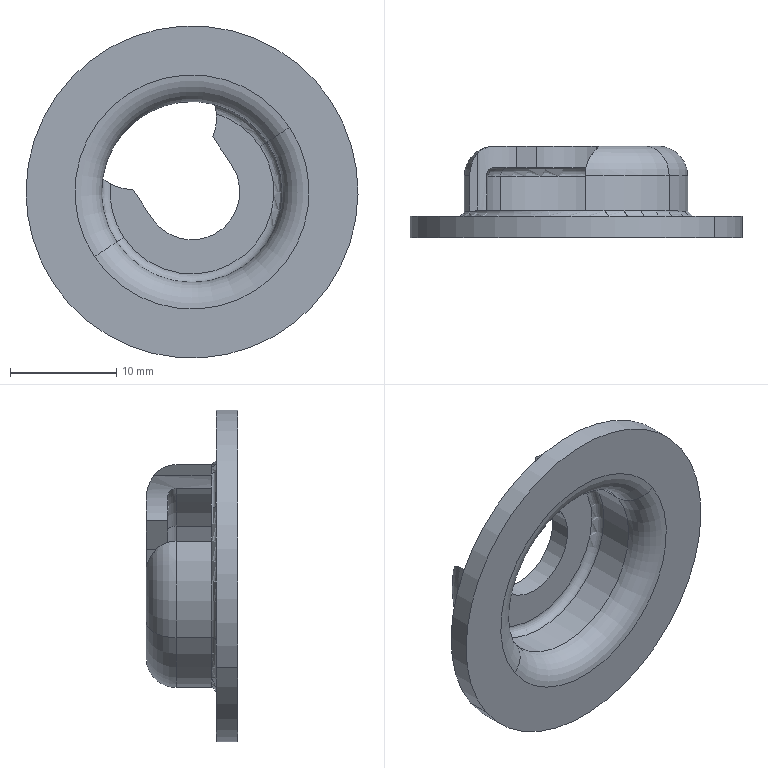Part | SolidWorks | features BaseBody 1 | 1 solid | 30 faces | box 31.2 x 8.6 x 31.2 mm | volume 1769 mm3 | cylinder 11 | torus 10 | plane 9 | commonest cylinder face diameters 9 x3 17 x3 21 x3 31.2 x2
STEP:
#1=CARTESIAN_POINT('',(45.671,49.147,6.074));
#2=VERTEX_POINT('',#1);
#3=CARTESIAN_POINT('',(27.329,49.147,-6.074));
#4=VERTEX_POINT('',#3);
#5=CARTESIAN_POINT('',(36.5,49.147,0.));
#6=DIRECTION('',(0.,1.,0.));
#7=DIRECTION('',(-0.8337,0.,-0.5522));
#8=AXIS2_PLACEMENT_3D('',#5,#6,#7);
#9=CIRCLE('',#8,11.);
#10=EDGE_CURVE('',#2,#4,#9,.T.);
#11=ORIENTED_EDGE('',*,*,#10,.F.);
#12=CARTESIAN_POINT('',(43.587,51.647,4.693));
#13=VERTEX_POINT('',#12);
#14=CARTESIAN_POINT('',(45.671,51.647,6.074));
#15=DIRECTION('',(0.5522,0.,-0.8337));
#16=DIRECTION('',(-0.8337,0.,-0.5522));
#17=AXIS2_PLACEMENT_3D('',#14,#15,#16);
#18=CIRCLE('',#17,2.5);
#19=EDGE_CURVE('',#2,#13,#18,.T.);
#20=ORIENTED_EDGE('',*,*,#19,.T.);
#21=CARTESIAN_POINT('',(29.413,51.647,-4.693));
#22=VERTEX_POINT('',#21);
#23=CARTESIAN_POINT('',(36.5,51.647,0.));
#24=DIRECTION('',(0.,-1.,0.));
#25=DIRECTION('',(-0.8337,0.,-0.5522));
#26=AXIS2_PLACEMENT_3D('',#23,#24,#25);
#27=CIRCLE('',#26,8.5);
#28=EDGE_CURVE('',#22,#13,#27,.T.);
#29=ORIENTED_EDGE('',*,*,#28,.F.);
#30=CARTESIAN_POINT('',(27.329,51.647,-6.074));
#31=DIRECTION('',(-0.5522,0.,0.8337));
#32=DIRECTION('',(0.8337,0.,0.5522));
#33=AXIS2_PLACEMENT_3D('',#30,#31,#32);
#34=CIRCLE('',#33,2.5);
#35=EDGE_CURVE('',#4,#22,#34,.T.);
#36=ORIENTED_EDGE('',*,*,#35,.F.);
#37=EDGE_LOOP('',(#11,#20,#29,#36));
#38=FACE_OUTER_BOUND('',#37,.T.);
#39=CARTESIAN_POINT('',(36.5,51.647,0.));
#40=DIRECTION('',(0.,-1.,0.));
#41=DIRECTION('',(-0.8337,0.,-0.5522));
#42=AXIS2_PLACEMENT_3D('',#39,#40,#41);
#43=TOROIDAL_SURFACE('',#42,11.,2.5);
#44=ADVANCED_FACE('',(#38),#43,.T.);
#45=CARTESIAN_POINT('',(45.671,51.147,6.074));
#46=VERTEX_POINT('',#45);
#47=CARTESIAN_POINT('',(27.329,51.147,-6.074));
#48=VERTEX_POINT('',#47);
#49=CARTESIAN_POINT('',(36.5,51.147,0.));
#50=DIRECTION('',(0.,-1.,0.));
#51=DIRECTION('',(-0.8337,0.,-0.5522));
#52=AXIS2_PLACEMENT_3D('',#49,#50,#51);
#53=CIRCLE('',#52,11.);
#54=EDGE_CURVE('',#46,#48,#53,.T.);
#55=ORIENTED_EDGE('',*,*,#54,.F.);
#56=CARTESIAN_POINT('',(45.254,51.647,5.798));
#57=VERTEX_POINT('',#56);
#58=CARTESIAN_POINT('',(45.671,51.647,6.074));
#59=DIRECTION('',(0.5522,0.,-0.8337));
#60=DIRECTION('',(-0.8337,0.,-0.5522));
#61=AXIS2_PLACEMENT_3D('',#58,#59,#60);
#62=CIRCLE('',#61,0.5);
#63=EDGE_CURVE('',#46,#57,#62,.T.);
#64=ORIENTED_EDGE('',*,*,#63,.T.);
#65=CARTESIAN_POINT('',(37.366,51.647,10.464));
#66=VERTEX_POINT('',#65);
#67=CARTESIAN_POINT('',(36.5,51.647,0.));
#68=DIRECTION('',(0.,1.,0.));
#69=DIRECTION('',(-0.8337,0.,-0.5522));
#70=AXIS2_PLACEMENT_3D('',#67,#68,#69);
#71=CIRCLE('',#70,10.5);
#72=EDGE_CURVE('',#66,#57,#71,.T.);
#73=ORIENTED_EDGE('',*,*,#72,.F.);
#74=CARTESIAN_POINT('',(26.527,51.647,3.286));
#75=VERTEX_POINT('',#74);
#76=CARTESIAN_POINT('',(36.5,51.647,0.));
#77=DIRECTION('',(0.,1.,0.));
#78=DIRECTION('',(-0.8337,0.,-0.5522));
#79=AXIS2_PLACEMENT_3D('',#76,#77,#78);
#80=CIRCLE('',#79,10.5);
#81=EDGE_CURVE('',#75,#66,#80,.T.);
#82=ORIENTED_EDGE('',*,*,#81,.F.);
#83=CARTESIAN_POINT('',(27.746,51.647,-5.798));
#84=VERTEX_POINT('',#83);
#85=CARTESIAN_POINT('',(36.5,51.647,0.));
#86=DIRECTION('',(0.,1.,0.));
#87=DIRECTION('',(-0.8337,0.,-0.5522));
#88=AXIS2_PLACEMENT_3D('',#85,#86,#87);
#89=CIRCLE('',#88,10.5);
#90=EDGE_CURVE('',#84,#75,#89,.T.);
#91=ORIENTED_EDGE('',*,*,#90,.F.);
#92=CARTESIAN_POINT('',(27.329,51.647,-6.074));
#93=DIRECTION('',(-0.5522,0.,0.8337));
#94=DIRECTION('',(0.8337,0.,0.5522));
#95=AXIS2_PLACEMENT_3D('',#92,#93,#94);
#96=CIRCLE('',#95,0.5);
#97=EDGE_CURVE('',#48,#84,#96,.T.);
#98=ORIENTED_EDGE('',*,*,#97,.F.);
#99=EDGE_LOOP('',(#55,#64,#73,#82,#91,#98));
#100=FACE_OUTER_BOUND('',#99,.T.);
#101=CARTESIAN_POINT('',(36.5,51.647,0.));
#102=DIRECTION('',(0.,-1.,0.));
#103=DIRECTION('',(-0.8337,0.,-0.5522));
#104=AXIS2_PLACEMENT_3D('',#101,#102,#103);
#105=TOROIDAL_SURFACE('',#104,11.,0.5);
#106=ADVANCED_FACE('',(#100),#105,.F.);
#107=CARTESIAN_POINT('',(42.92,57.747,4.252));
#108=VERTEX_POINT('',#107);
#109=CARTESIAN_POINT('',(30.08,57.747,-4.252));
#110=VERTEX_POINT('',#109);
#111=CARTESIAN_POINT('',(36.5,57.747,0.));
#112=DIRECTION('',(0.,1.,0.));
#113=DIRECTION('',(-0.8337,0.,-0.5522));
#114=AXIS2_PLACEMENT_3D('',#111,#112,#113);
#115=CIRCLE('',#114,7.7);
#116=EDGE_CURVE('',#108,#110,#115,.T.);
#117=ORIENTED_EDGE('',*,*,#116,.F.);
#118=CARTESIAN_POINT('',(45.254,54.947,5.798));
#119=VERTEX_POINT('',#118);
#120=CARTESIAN_POINT('',(42.92,54.947,4.252));
#121=DIRECTION('',(0.5522,0.,-0.8337));
#122=DIRECTION('',(-0.8337,0.,-0.5522));
#123=AXIS2_PLACEMENT_3D('',#120,#121,#122);
#124=CIRCLE('',#123,2.8);
#125=EDGE_CURVE('',#108,#119,#124,.T.);
#126=ORIENTED_EDGE('',*,*,#125,.T.);
#127=CARTESIAN_POINT('',(27.746,54.947,-5.798));
#128=VERTEX_POINT('',#127);
#129=CARTESIAN_POINT('',(36.5,54.947,0.));
#130=DIRECTION('',(0.,-1.,0.));
#131=DIRECTION('',(-0.8337,0.,-0.5522));
#132=AXIS2_PLACEMENT_3D('',#129,#130,#131);
#133=CIRCLE('',#132,10.5);
#134=EDGE_CURVE('',#128,#119,#133,.T.);
#135=ORIENTED_EDGE('',*,*,#134,.F.);
#136=CARTESIAN_POINT('',(30.08,54.947,-4.252));
#137=DIRECTION('',(-0.5522,0.,0.8337));
#138=DIRECTION('',(0.8337,0.,0.5522));
#139=AXIS2_PLACEMENT_3D('',#136,#137,#138);
#140=CIRCLE('',#139,2.8);
#141=EDGE_CURVE('',#110,#128,#140,.T.);
#142=ORIENTED_EDGE('',*,*,#141,.F.);
#143=EDGE_LOOP('',(#117,#126,#135,#142));
#144=FACE_OUTER_BOUND('',#143,.T.);
#145=CARTESIAN_POINT('',(36.5,54.947,0.));
#146=DIRECTION('',(0.,-1.,0.));
#147=DIRECTION('',(-0.8337,0.,-0.5522));
#148=AXIS2_PLACEMENT_3D('',#145,#146,#147);
#149=TOROIDAL_SURFACE('',#148,7.7,2.8);
#150=ADVANCED_FACE('',(#144),#149,.T.);
#151=CARTESIAN_POINT('',(28.838,57.747,0.7673));
#152=VERTEX_POINT('',#151);
#153=CARTESIAN_POINT('',(36.5,57.747,0.));
#154=DIRECTION('',(0.,1.,0.));
#155=DIRECTION('',(-0.8337,0.,-0.5522));
#156=AXIS2_PLACEMENT_3D('',#153,#154,#155);
#157=CIRCLE('',#156,7.7);
#158=EDGE_CURVE('',#110,#152,#157,.T.);
#159=ORIENTED_EDGE('',*,*,#158,.F.);
#160=ORIENTED_EDGE('',*,*,#141,.T.);
#161=CARTESIAN_POINT('',(26.527,54.947,3.286));
#162=VERTEX_POINT('',#161);
#163=CARTESIAN_POINT('',(36.5,54.947,0.));
#164=DIRECTION('',(0.,-1.,0.));
#165=DIRECTION('',(-0.8337,0.,-0.5522));
#166=AXIS2_PLACEMENT_3D('',#163,#164,#165);
#167=CIRCLE('',#166,10.5);
#168=EDGE_CURVE('',#162,#128,#167,.T.);
#169=ORIENTED_EDGE('',*,*,#168,.F.);
#170=CARTESIAN_POINT('',(27.216,57.047,2.247));
#171=VERTEX_POINT('',#170);
#172=CARTESIAN_POINT('',(27.216,57.047,2.247));
#173=CARTESIAN_POINT('',(27.116,56.93,2.397));
#174=CARTESIAN_POINT('',(27.024,56.799,2.536));
#175=CARTESIAN_POINT('',(26.858,56.501,2.788));
#176=CARTESIAN_POINT('',(26.782,56.333,2.901));
#177=CARTESIAN_POINT('',(26.658,55.969,3.088));
#178=CARTESIAN_POINT('',(26.61,55.774,3.162));
#179=CARTESIAN_POINT('',(26.545,55.37,3.26));
#180=CARTESIAN_POINT('',(26.527,55.157,3.286));
#181=CARTESIAN_POINT('',(26.527,54.947,3.286));
#182=B_SPLINE_CURVE_WITH_KNOTS('',3,(#172,#173,#174,#175,#176,#177,#178,#179,#180,#181),.UNSPECIFIED.,.F.,.F.,(4,2,2,2,4),(0.03709,0.03772,0.03835,0.03898,0.03961),.UNSPECIFIED.);
#183=EDGE_CURVE('',#171,#162,#182,.T.);
#184=ORIENTED_EDGE('',*,*,#183,.F.);
#185=CARTESIAN_POINT('',(28.838,57.747,0.7673));
#186=CARTESIAN_POINT('',(28.665,57.747,0.8605));
#187=CARTESIAN_POINT('',(28.498,57.729,0.9649));
#188=CARTESIAN_POINT('',(28.185,57.664,1.19));
#189=CARTESIAN_POINT('',(28.036,57.615,1.313));
#190=CARTESIAN_POINT('',(27.627,57.433,1.694));
#191=CARTESIAN_POINT('',(27.399,57.261,1.97));
#192=CARTESIAN_POINT('',(27.216,57.047,2.247));
#193=B_SPLINE_CURVE_WITH_KNOTS('',3,(#185,#186,#187,#188,#189,#190,#191,#192),.UNSPECIFIED.,.F.,.F.,(4,2,2,4),(0.002486,0.003072,0.003657,0.004829),.UNSPECIFIED.);
#194=EDGE_CURVE('',#152,#171,#193,.T.);
#195=ORIENTED_EDGE('',*,*,#194,.F.);
#196=EDGE_LOOP('',(#159,#160,#169,#184,#195));
#197=FACE_OUTER_BOUND('',#196,.T.);
#198=CARTESIAN_POINT('',(36.5,54.947,0.));
#199=DIRECTION('',(0.,-1.,0.));
#200=DIRECTION('',(-0.8337,0.,-0.5522));
#201=AXIS2_PLACEMENT_3D('',#198,#199,#200);
#202=TOROIDAL_SURFACE('',#201,7.7,2.8);
#203=ADVANCED_FACE('',(#197),#202,.T.);
#204=CARTESIAN_POINT('',(29.413,54.947,-4.693));
#205=VERTEX_POINT('',#204);
#206=CARTESIAN_POINT('',(28.095,54.947,1.268));
#207=VERTEX_POINT('',#206);
#208=CARTESIAN_POINT('',(36.5,54.947,0.));
#209=DIRECTION('',(0.,1.,0.));
#210=DIRECTION('',(0.8337,0.,0.5522));
#211=AXIS2_PLACEMENT_3D('',#208,#209,#210);
#212=CIRCLE('',#211,8.5);
#213=EDGE_CURVE('',#205,#207,#212,.T.);
#214=ORIENTED_EDGE('',*,*,#213,.F.);
#215=CARTESIAN_POINT('',(30.08,55.747,-4.252));
#216=VERTEX_POINT('',#215);
#217=CARTESIAN_POINT('',(30.08,54.947,-4.252));
#218=DIRECTION('',(0.5522,0.,-0.8337));
#219=DIRECTION('',(-0.8337,0.,-0.5522));
#220=AXIS2_PLACEMENT_3D('',#217,#218,#219);
#221=CIRCLE('',#220,0.8);
#222=EDGE_CURVE('',#205,#216,#221,.T.);
#223=ORIENTED_EDGE('',*,*,#222,.T.);
#224=CARTESIAN_POINT('',(28.838,55.747,0.7673));
#225=VERTEX_POINT('',#224);
#226=CARTESIAN_POINT('',(36.5,55.747,0.));
#227=DIRECTION('',(0.,-1.,0.));
#228=DIRECTION('',(0.8337,0.,0.5522));
#229=AXIS2_PLACEMENT_3D('',#226,#227,#228);
#230=CIRCLE('',#229,7.7);
#231=EDGE_CURVE('',#225,#216,#230,.T.);
#232=ORIENTED_EDGE('',*,*,#231,.F.);
#233=CARTESIAN_POINT('',(28.838,55.747,0.7673));
#234=CARTESIAN_POINT('',(28.74,55.747,0.8198));
#235=CARTESIAN_POINT('',(28.645,55.728,0.8757));
#236=CARTESIAN_POINT('',(28.468,55.652,0.988));
#237=CARTESIAN_POINT('',(28.389,55.597,1.043));
#238=CARTESIAN_POINT('',(28.251,55.453,1.143));
#239=CARTESIAN_POINT('',(28.195,55.368,1.187));
#240=CARTESIAN_POINT('',(28.116,55.168,1.25));
#241=CARTESIAN_POINT('',(28.095,55.059,1.268));
#242=CARTESIAN_POINT('',(28.095,54.947,1.268));
#243=B_SPLINE_CURVE_WITH_KNOTS('',3,(#233,#234,#235,#236,#237,#238,#239,#240,#241,#242),.UNSPECIFIED.,.F.,.F.,(4,2,2,2,4),(0.001287,0.001619,0.00195,0.002281,0.002613),.UNSPECIFIED.);
#244=EDGE_CURVE('',#225,#207,#243,.T.);
#245=ORIENTED_EDGE('',*,*,#244,.T.);
#246=EDGE_LOOP('',(#214,#223,#232,#245));
#247=FACE_OUTER_BOUND('',#246,.T.);
#248=CARTESIAN_POINT('',(36.5,54.947,0.));
#249=DIRECTION('',(0.,1.,0.));
#250=DIRECTION('',(0.8337,0.,0.5522));
#251=AXIS2_PLACEMENT_3D('',#248,#249,#250);
#252=TOROIDAL_SURFACE('',#251,7.7,0.8);
#253=ADVANCED_FACE('',(#247),#252,.F.);
#254=ORIENTED_EDGE('',*,*,#222,.F.);
#255=CARTESIAN_POINT('',(43.587,54.947,4.693));
#256=VERTEX_POINT('',#255);
#257=CARTESIAN_POINT('',(36.5,54.947,0.));
#258=DIRECTION('',(0.,1.,0.));
#259=DIRECTION('',(0.8337,0.,0.5522));
#260=AXIS2_PLACEMENT_3D('',#257,#258,#259);
#261=CIRCLE('',#260,8.5);
#262=EDGE_CURVE('',#256,#205,#261,.T.);
#263=ORIENTED_EDGE('',*,*,#262,.F.);
#264=CARTESIAN_POINT('',(42.92,55.747,4.252));
#265=VERTEX_POINT('',#264);
#266=CARTESIAN_POINT('',(42.92,54.947,4.252));
#267=DIRECTION('',(-0.5522,0.,0.8337));
#268=DIRECTION('',(0.8337,0.,0.5522));
#269=AXIS2_PLACEMENT_3D('',#266,#267,#268);
#270=CIRCLE('',#269,0.8);
#271=EDGE_CURVE('',#256,#265,#270,.T.);
#272=ORIENTED_EDGE('',*,*,#271,.T.);
#273=CARTESIAN_POINT('',(36.5,55.747,0.));
#274=DIRECTION('',(0.,-1.,0.));
#275=DIRECTION('',(0.8337,0.,0.5522));
#276=AXIS2_PLACEMENT_3D('',#273,#274,#275);
#277=CIRCLE('',#276,7.7);
#278=EDGE_CURVE('',#216,#265,#277,.T.);
#279=ORIENTED_EDGE('',*,*,#278,.F.);
#280=EDGE_LOOP('',(#254,#263,#272,#279));
#281=FACE_OUTER_BOUND('',#280,.T.);
#282=CARTESIAN_POINT('',(36.5,54.947,0.));
#283=DIRECTION('',(0.,1.,0.));
#284=DIRECTION('',(0.8337,0.,0.5522));
#285=AXIS2_PLACEMENT_3D('',#282,#283,#284);
#286=TOROIDAL_SURFACE('',#285,7.7,0.8);
#287=ADVANCED_FACE('',(#281),#286,.F.);
#288=CARTESIAN_POINT('',(38.613,54.947,8.233));
#289=VERTEX_POINT('',#288);
#290=CARTESIAN_POINT('',(36.5,54.947,0.));
#291=DIRECTION('',(0.,1.,0.));
#292=DIRECTION('',(0.8337,0.,0.5522));
#293=AXIS2_PLACEMENT_3D('',#290,#291,#292);
#294=CIRCLE('',#293,8.5);
#295=EDGE_CURVE('',#289,#256,#294,.T.);
#296=ORIENTED_EDGE('',*,*,#295,.T.);
#297=CARTESIAN_POINT('',(43.587,55.747,4.693));
#298=DIRECTION('',(0.,-1.,0.));
#299=VECTOR('',#298,1000.);
#300=LINE('',#297,#299);
#301=EDGE_CURVE('',#256,#13,#300,.T.);
#302=ORIENTED_EDGE('',*,*,#301,.T.);
#303=CARTESIAN_POINT('',(38.613,51.647,8.233));
#304=VERTEX_POINT('',#303);
#305=CARTESIAN_POINT('',(36.5,51.647,0.));
#306=DIRECTION('',(0.,-1.,0.));
#307=DIRECTION('',(-0.8337,0.,-0.5522));
#308=AXIS2_PLACEMENT_3D('',#305,#306,#307);
#309=CIRCLE('',#308,8.5);
#310=EDGE_CURVE('',#13,#304,#309,.T.);
#311=ORIENTED_EDGE('',*,*,#310,.T.);
#312=CARTESIAN_POINT('',(38.613,54.697,8.233));
#313=DIRECTION('',(0.,-1.,0.));
#314=VECTOR('',#313,1000.);
#315=LINE('',#312,#314);
#316=EDGE_CURVE('',#289,#304,#315,.T.);
#317=ORIENTED_EDGE('',*,*,#316,.F.);
#318=EDGE_LOOP('',(#296,#302,#311,#317));
#319=FACE_OUTER_BOUND('',#318,.T.);
#320=CARTESIAN_POINT('',(36.5,55.747,0.));
#321=DIRECTION('',(0.,-1.,0.));
#322=DIRECTION('',(-0.8337,0.,-0.5522));
#323=AXIS2_PLACEMENT_3D('',#320,#321,#322);
#324=CYLINDRICAL_SURFACE('',#323,8.5);
#325=ADVANCED_FACE('',(#319),#324,.F.);
#326=ORIENTED_EDGE('',*,*,#301,.F.);
#327=ORIENTED_EDGE('',*,*,#262,.T.);
#328=CARTESIAN_POINT('',(29.413,55.747,-4.693));
#329=DIRECTION('',(0.,-1.,0.));
#330=VECTOR('',#329,1000.);
#331=LINE('',#328,#330);
#332=EDGE_CURVE('',#205,#22,#331,.T.);
#333=ORIENTED_EDGE('',*,*,#332,.T.);
#334=ORIENTED_EDGE('',*,*,#28,.T.);
#335=EDGE_LOOP('',(#326,#327,#333,#334));
#336=FACE_OUTER_BOUND('',#335,.T.);
#337=CARTESIAN_POINT('',(36.5,55.747,0.));
#338=DIRECTION('',(0.,-1.,0.));
#339=DIRECTION('',(-0.8337,0.,-0.5522));
#340=AXIS2_PLACEMENT_3D('',#337,#338,#339);
#341=CYLINDRICAL_SURFACE('',#340,8.5);
#342=ADVANCED_FACE('',(#336),#341,.F.);
#343=CARTESIAN_POINT('',(23.494,51.147,-8.614));
#344=VERTEX_POINT('',#343);
#345=CARTESIAN_POINT('',(49.506,51.147,8.614));
#346=VERTEX_POINT('',#345);
#347=CARTESIAN_POINT('',(36.5,51.147,0.));
#348=DIRECTION('',(0.,-1.,0.));
#349=DIRECTION('',(-0.8337,0.,-0.5522));
#350=AXIS2_PLACEMENT_3D('',#347,#348,#349);
#351=CIRCLE('',#350,15.6);
#352=EDGE_CURVE('',#344,#346,#351,.T.);
#353=ORIENTED_EDGE('',*,*,#352,.T.);
#354=CARTESIAN_POINT('',(49.506,49.147,8.614));
#355=VERTEX_POINT('',#354);
#356=CARTESIAN_POINT('',(49.506,51.147,8.614));
#357=DIRECTION('',(0.,-1.,0.));
#358=VECTOR('',#357,1000.);
#359=LINE('',#356,#358);
#360=EDGE_CURVE('',#346,#355,#359,.T.);
#361=ORIENTED_EDGE('',*,*,#360,.T.);
#362=CARTESIAN_POINT('',(23.494,49.147,-8.614));
#363=VERTEX_POINT('',#362);
#364=CARTESIAN_POINT('',(36.5,49.147,0.));
#365=DIRECTION('',(0.,-1.,0.));
#366=DIRECTION('',(-0.8337,0.,-0.5522));
#367=AXIS2_PLACEMENT_3D('',#364,#365,#366);
#368=CIRCLE('',#367,15.6);
#369=EDGE_CURVE('',#363,#355,#368,.T.);
#370=ORIENTED_EDGE('',*,*,#369,.F.);
#371=CARTESIAN_POINT('',(23.494,51.147,-8.614));
#372=DIRECTION('',(0.,-1.,0.));
#373=VECTOR('',#372,1000.);
#374=LINE('',#371,#373);
#375=EDGE_CURVE('',#344,#363,#374,.T.);
#376=ORIENTED_EDGE('',*,*,#375,.F.);
#377=EDGE_LOOP('',(#353,#361,#370,#376));
#378=FACE_OUTER_BOUND('',#377,.T.);
#379=CARTESIAN_POINT('',(36.5,51.147,0.));
#380=DIRECTION('',(0.,-1.,0.));
#381=DIRECTION('',(-0.8337,0.,-0.5522));
#382=AXIS2_PLACEMENT_3D('',#379,#380,#381);
#383=CYLINDRICAL_SURFACE('',#382,15.6);
#384=ADVANCED_FACE('',(#378),#383,.T.);
#385=CARTESIAN_POINT('',(36.5,51.647,0.));
#386=DIRECTION('',(0.,1.,0.));
#387=DIRECTION('',(-0.8337,0.,-0.5522));
#388=AXIS2_PLACEMENT_3D('',#385,#386,#387);
#389=CIRCLE('',#388,10.5);
#390=EDGE_CURVE('',#57,#84,#389,.T.);
#391=ORIENTED_EDGE('',*,*,#390,.T.);
#392=CARTESIAN_POINT('',(27.746,49.147,-5.798));
#393=DIRECTION('',(0.,1.,0.));
#394=VECTOR('',#393,1000.);
#395=LINE('',#392,#394);
#396=EDGE_CURVE('',#84,#128,#395,.T.);
#397=ORIENTED_EDGE('',*,*,#396,.T.);
#398=ORIENTED_EDGE('',*,*,#134,.T.);
#399=CARTESIAN_POINT('',(45.254,49.147,5.798));
#400=DIRECTION('',(0.,1.,0.));
#401=VECTOR('',#400,1000.);
#402=LINE('',#399,#401);
#403=EDGE_CURVE('',#57,#119,#402,.T.);
#404=ORIENTED_EDGE('',*,*,#403,.F.);
#405=EDGE_LOOP('',(#391,#397,#398,#404));
#406=FACE_OUTER_BOUND('',#405,.T.);
#407=CARTESIAN_POINT('',(36.5,49.147,0.));
#408=DIRECTION('',(0.,1.,0.));
#409=DIRECTION('',(0.8337,0.,0.5522));
#410=AXIS2_PLACEMENT_3D('',#407,#408,#409);
#411=CYLINDRICAL_SURFACE('',#410,10.5);
#412=ADVANCED_FACE('',(#406),#411,.T.);
#413=ORIENTED_EDGE('',*,*,#72,.T.);
#414=ORIENTED_EDGE('',*,*,#403,.T.);
#415=CARTESIAN_POINT('',(37.366,54.947,10.464));
#416=VERTEX_POINT('',#415);
#417=CARTESIAN_POINT('',(36.5,54.947,0.));
#418=DIRECTION('',(0.,-1.,0.));
#419=DIRECTION('',(-0.8337,0.,-0.5522));
#420=AXIS2_PLACEMENT_3D('',#417,#418,#419);
#421=CIRCLE('',#420,10.5);
#422=EDGE_CURVE('',#119,#416,#421,.T.);
#423=ORIENTED_EDGE('',*,*,#422,.T.);
#424=CARTESIAN_POINT('',(37.366,49.147,10.464));
#425=DIRECTION('',(0.,-1.,0.));
#426=VECTOR('',#425,1000.);
#427=LINE('',#424,#426);
#428=EDGE_CURVE('',#416,#66,#427,.T.);
#429=ORIENTED_EDGE('',*,*,#428,.T.);
#430=EDGE_LOOP('',(#413,#414,#423,#429));
#431=FACE_OUTER_BOUND('',#430,.T.);
#432=CARTESIAN_POINT('',(36.5,49.147,0.));
#433=DIRECTION('',(0.,1.,0.));
#434=DIRECTION('',(0.8337,0.,0.5522));
#435=AXIS2_PLACEMENT_3D('',#432,#433,#434);
#436=CYLINDRICAL_SURFACE('',#435,10.5);
#437=ADVANCED_FACE('',(#431),#436,.T.);
#438=CARTESIAN_POINT('',(36.5,49.147,0.));
#439=DIRECTION('',(0.,1.,0.));
#440=DIRECTION('',(-0.8337,0.,-0.5522));
#441=AXIS2_PLACEMENT_3D('',#438,#439,#440);
#442=CIRCLE('',#441,11.);
#443=EDGE_CURVE('',#4,#2,#442,.T.);
#444=ORIENTED_EDGE('',*,*,#443,.T.);
#445=ORIENTED_EDGE('',*,*,#10,.T.);
#446=EDGE_LOOP('',(#444,#445));
#447=FACE_BOUND('',#446,.T.);
#448=ORIENTED_EDGE('',*,*,#369,.T.);
#449=CARTESIAN_POINT('',(36.5,49.147,0.));
#450=DIRECTION('',(0.,-1.,0.));
#451=DIRECTION('',(-0.8337,0.,-0.5522));
#452=AXIS2_PLACEMENT_3D('',#449,#450,#451);
#453=CIRCLE('',#452,15.6);
#454=EDGE_CURVE('',#355,#363,#453,.T.);
#455=ORIENTED_EDGE('',*,*,#454,.T.);
#456=EDGE_LOOP('',(#448,#455));
#457=FACE_OUTER_BOUND('',#456,.T.);
#458=CARTESIAN_POINT('',(36.5,49.147,0.));
#459=DIRECTION('',(0.,-1.,0.));
#460=DIRECTION('',(-0.8337,0.,-0.5522));
#461=AXIS2_PLACEMENT_3D('',#458,#459,#460);
#462=PLANE('',#461);
#463=ADVANCED_FACE('',(#447,#457),#462,.T.);
#464=ORIENTED_EDGE('',*,*,#396,.F.);
#465=ORIENTED_EDGE('',*,*,#90,.T.);
#466=CARTESIAN_POINT('',(26.527,49.147,3.286));
#467=DIRECTION('',(0.,1.,0.));
#468=VECTOR('',#467,1000.);
#469=LINE('',#466,#468);
#470=EDGE_CURVE('',#75,#162,#469,.T.);
#471=ORIENTED_EDGE('',*,*,#470,.T.);
#472=ORIENTED_EDGE('',*,*,#168,.T.);
#473=EDGE_LOOP('',(#464,#465,#471,#472));
#474=FACE_OUTER_BOUND('',#473,.T.);
#475=CARTESIAN_POINT('',(36.5,49.147,0.));
#476=DIRECTION('',(0.,1.,0.));
#477=DIRECTION('',(0.8337,0.,0.5522));
#478=AXIS2_PLACEMENT_3D('',#475,#476,#477);
#479=CYLINDRICAL_SURFACE('',#478,10.5);
#480=ADVANCED_FACE('',(#474),#479,.T.);
#481=CARTESIAN_POINT('',(30.949,57.747,0.2318));
#482=VERTEX_POINT('',#481);
#483=CARTESIAN_POINT('',(30.967,57.747,4.732));
#484=DIRECTION('',(0.,1.,0.));
#485=DIRECTION('',(0.8337,0.,0.5522));
#486=AXIS2_PLACEMENT_3D('',#483,#484,#485);
#487=CIRCLE('',#486,4.5);
#488=EDGE_CURVE('',#482,#152,#487,.T.);
#489=ORIENTED_EDGE('',*,*,#488,.F.);
#490=CARTESIAN_POINT('',(32.748,57.747,-2.485));
#491=VERTEX_POINT('',#490);
#492=CARTESIAN_POINT('',(32.748,57.747,-2.485));
#493=DIRECTION('',(-0.5522,0.,0.8337));
#494=VECTOR('',#493,1000.);
#495=LINE('',#492,#494);
#496=EDGE_CURVE('',#491,#482,#495,.T.);
#497=ORIENTED_EDGE('',*,*,#496,.F.);
#498=CARTESIAN_POINT('',(40.252,57.747,2.485));
#499=VERTEX_POINT('',#498);
#500=CARTESIAN_POINT('',(36.5,57.747,0.));
#501=DIRECTION('',(0.,1.,0.));
#502=DIRECTION('',(0.8337,0.,0.5522));
#503=AXIS2_PLACEMENT_3D('',#500,#501,#502);
#504=CIRCLE('',#503,4.5);
#505=EDGE_CURVE('',#499,#491,#504,.T.);
#506=ORIENTED_EDGE('',*,*,#505,.F.);
#507=CARTESIAN_POINT('',(38.453,57.747,5.201));
#508=VERTEX_POINT('',#507);
#509=CARTESIAN_POINT('',(40.252,57.747,2.485));
#510=DIRECTION('',(0.5522,0.,-0.8337));
#511=VECTOR('',#510,1000.);
#512=LINE('',#509,#511);
#513=EDGE_CURVE('',#508,#499,#512,.T.);
#514=ORIENTED_EDGE('',*,*,#513,.F.);
#515=CARTESIAN_POINT('',(38.783,57.747,7.354));
#516=VERTEX_POINT('',#515);
#517=CARTESIAN_POINT('',(34.302,57.747,6.94));
#518=DIRECTION('',(0.,1.,0.));
#519=DIRECTION('',(-0.8337,0.,-0.5522));
#520=AXIS2_PLACEMENT_3D('',#517,#518,#519);
#521=CIRCLE('',#520,4.5);
#522=EDGE_CURVE('',#516,#508,#521,.T.);
#523=ORIENTED_EDGE('',*,*,#522,.F.);
#524=CARTESIAN_POINT('',(36.5,57.747,0.));
#525=DIRECTION('',(0.,1.,0.));
#526=DIRECTION('',(-0.8337,0.,-0.5522));
#527=AXIS2_PLACEMENT_3D('',#524,#525,#526);
#528=CIRCLE('',#527,7.7);
#529=EDGE_CURVE('',#516,#108,#528,.T.);
#530=ORIENTED_EDGE('',*,*,#529,.T.);
#531=ORIENTED_EDGE('',*,*,#116,.T.);
#532=ORIENTED_EDGE('',*,*,#158,.T.);
#533=EDGE_LOOP('',(#489,#497,#506,#514,#523,#530,#531,#532));
#534=FACE_OUTER_BOUND('',#533,.T.);
#535=CARTESIAN_POINT('',(36.5,57.747,0.));
#536=DIRECTION('',(0.,-1.,0.));
#537=DIRECTION('',(-0.8337,0.,-0.5522));
#538=AXIS2_PLACEMENT_3D('',#535,#536,#537);
#539=PLANE('',#538);
#540=ADVANCED_FACE('',(#534),#539,.F.);
#541=CARTESIAN_POINT('',(36.5,51.147,0.));
#542=DIRECTION('',(0.,-1.,0.));
#543=DIRECTION('',(-0.8337,0.,-0.5522));
#544=AXIS2_PLACEMENT_3D('',#541,#542,#543);
#545=CIRCLE('',#544,11.);
#546=EDGE_CURVE('',#48,#46,#545,.T.);
#547=ORIENTED_EDGE('',*,*,#546,.T.);
#548=ORIENTED_EDGE('',*,*,#54,.T.);
#549=EDGE_LOOP('',(#547,#548));
#550=FACE_BOUND('',#549,.T.);
#551=ORIENTED_EDGE('',*,*,#352,.F.);
#552=CARTESIAN_POINT('',(36.5,51.147,0.));
#553=DIRECTION('',(0.,-1.,0.));
#554=DIRECTION('',(-0.8337,0.,-0.5522));
#555=AXIS2_PLACEMENT_3D('',#552,#553,#554);
#556=CIRCLE('',#555,15.6);
#557=EDGE_CURVE('',#346,#344,#556,.T.);
#558=ORIENTED_EDGE('',*,*,#557,.F.);
#559=EDGE_LOOP('',(#551,#558));
#560=FACE_OUTER_BOUND('',#559,.T.);
#561=CARTESIAN_POINT('',(36.5,51.147,0.));
#562=DIRECTION('',(0.,-1.,0.));
#563=DIRECTION('',(-0.8337,0.,-0.5522));
#564=AXIS2_PLACEMENT_3D('',#561,#562,#563);
#565=PLANE('',#564);
#566=ADVANCED_FACE('',(#550,#560),#565,.F.);
#567=ORIENTED_EDGE('',*,*,#360,.F.);
#568=ORIENTED_EDGE('',*,*,#557,.T.);
#569=ORIENTED_EDGE('',*,*,#375,.T.);
#570=ORIENTED_EDGE('',*,*,#454,.F.);
#571=EDGE_LOOP('',(#567,#568,#569,#570));
#572=FACE_OUTER_BOUND('',#571,.T.);
#573=CARTESIAN_POINT('',(36.5,51.147,0.));
#574=DIRECTION('',(0.,-1.,0.));
#575=DIRECTION('',(-0.8337,0.,-0.5522));
#576=AXIS2_PLACEMENT_3D('',#573,#574,#575);
#577=CYLINDRICAL_SURFACE('',#576,15.6);
#578=ADVANCED_FACE('',(#572),#577,.T.);
#579=ORIENTED_EDGE('',*,*,#332,.F.);
#580=ORIENTED_EDGE('',*,*,#213,.T.);
#581=CARTESIAN_POINT('',(28.095,51.647,1.268));
#582=VERTEX_POINT('',#581);
#583=CARTESIAN_POINT('',(28.095,54.697,1.268));
#584=DIRECTION('',(0.,1.,0.));
#585=VECTOR('',#584,1000.);
#586=LINE('',#583,#585);
#587=EDGE_CURVE('',#582,#207,#586,.T.);
#588=ORIENTED_EDGE('',*,*,#587,.F.);
#589=CARTESIAN_POINT('',(36.5,51.647,0.));
#590=DIRECTION('',(0.,-1.,0.));
#591=DIRECTION('',(-0.8337,0.,-0.5522));
#592=AXIS2_PLACEMENT_3D('',#589,#590,#591);
#593=CIRCLE('',#592,8.5);
#594=EDGE_CURVE('',#582,#22,#593,.T.);
#595=ORIENTED_EDGE('',*,*,#594,.T.);
#596=EDGE_LOOP('',(#579,#580,#588,#595));
#597=FACE_OUTER_BOUND('',#596,.T.);
#598=CARTESIAN_POINT('',(36.5,55.747,0.));
#599=DIRECTION('',(0.,-1.,0.));
#600=DIRECTION('',(-0.8337,0.,-0.5522));
#601=AXIS2_PLACEMENT_3D('',#598,#599,#600);
#602=CYLINDRICAL_SURFACE('',#601,8.5);
#603=ADVANCED_FACE('',(#597),#602,.F.);
#604=CARTESIAN_POINT('',(40.252,55.747,2.485));
#605=VERTEX_POINT('',#604);
#606=CARTESIAN_POINT('',(32.748,55.747,-2.485));
#607=VERTEX_POINT('',#606);
#608=CARTESIAN_POINT('',(36.5,55.747,0.));
#609=DIRECTION('',(0.,1.,0.));
#610=DIRECTION('',(0.8337,0.,0.5522));
#611=AXIS2_PLACEMENT_3D('',#608,#609,#610);
#612=CIRCLE('',#611,4.5);
#613=EDGE_CURVE('',#605,#607,#612,.T.);
#614=ORIENTED_EDGE('',*,*,#613,.T.);
#615=CARTESIAN_POINT('',(30.949,55.747,0.2318));
#616=VERTEX_POINT('',#615);
#617=CARTESIAN_POINT('',(32.748,55.747,-2.485));
#618=DIRECTION('',(-0.5522,0.,0.8337));
#619=VECTOR('',#618,1000.);
#620=LINE('',#617,#619);
#621=EDGE_CURVE('',#607,#616,#620,.T.);
#622=ORIENTED_EDGE('',*,*,#621,.T.);
#623=CARTESIAN_POINT('',(30.967,55.747,4.732));
#624=DIRECTION('',(0.,1.,0.));
#625=DIRECTION('',(0.8337,0.,0.5522));
#626=AXIS2_PLACEMENT_3D('',#623,#624,#625);
#627=CIRCLE('',#626,4.5);
#628=EDGE_CURVE('',#616,#225,#627,.T.);
#629=ORIENTED_EDGE('',*,*,#628,.T.);
#630=ORIENTED_EDGE('',*,*,#231,.T.);
#631=ORIENTED_EDGE('',*,*,#278,.T.);
#632=CARTESIAN_POINT('',(38.783,55.747,7.354));
#633=VERTEX_POINT('',#632);
#634=CARTESIAN_POINT('',(36.5,55.747,0.));
#635=DIRECTION('',(0.,-1.,0.));
#636=DIRECTION('',(0.8337,0.,0.5522));
#637=AXIS2_PLACEMENT_3D('',#634,#635,#636);
#638=CIRCLE('',#637,7.7);
#639=EDGE_CURVE('',#265,#633,#638,.T.);
#640=ORIENTED_EDGE('',*,*,#639,.T.);
#641=CARTESIAN_POINT('',(38.453,55.747,5.201));
#642=VERTEX_POINT('',#641);
#643=CARTESIAN_POINT('',(34.302,55.747,6.94));
#644=DIRECTION('',(0.,1.,0.));
#645=DIRECTION('',(0.8337,0.,0.5522));
#646=AXIS2_PLACEMENT_3D('',#643,#644,#645);
#647=CIRCLE('',#646,4.5);
#648=EDGE_CURVE('',#633,#642,#647,.T.);
#649=ORIENTED_EDGE('',*,*,#648,.T.);
#650=CARTESIAN_POINT('',(40.252,55.747,2.485));
#651=DIRECTION('',(0.5522,0.,-0.8337));
#652=VECTOR('',#651,1000.);
#653=LINE('',#650,#652);
#654=EDGE_CURVE('',#642,#605,#653,.T.);
#655=ORIENTED_EDGE('',*,*,#654,.T.);
#656=EDGE_LOOP('',(#614,#622,#629,#630,#631,#640,#649,#655));
#657=FACE_OUTER_BOUND('',#656,.T.);
#658=CARTESIAN_POINT('',(36.5,55.747,0.));
#659=DIRECTION('',(0.,1.,0.));
#660=DIRECTION('',(0.8337,0.,0.5522));
#661=AXIS2_PLACEMENT_3D('',#658,#659,#660);
#662=PLANE('',#661);
#663=ADVANCED_FACE('',(#657),#662,.F.);
#664=ORIENTED_EDGE('',*,*,#271,.F.);
#665=ORIENTED_EDGE('',*,*,#295,.F.);
#666=CARTESIAN_POINT('',(38.613,54.947,8.233));
#667=CARTESIAN_POINT('',(38.613,55.059,8.233));
#668=CARTESIAN_POINT('',(38.621,55.169,8.207));
#669=CARTESIAN_POINT('',(38.648,55.366,8.11));
#670=CARTESIAN_POINT('',(38.666,55.454,8.041));
#671=CARTESIAN_POINT('',(38.705,55.597,7.875));
#672=CARTESIAN_POINT('',(38.725,55.652,7.78));
#673=CARTESIAN_POINT('',(38.759,55.728,7.573));
#674=CARTESIAN_POINT('',(38.773,55.747,7.465));
#675=CARTESIAN_POINT('',(38.783,55.747,7.354));
#676=B_SPLINE_CURVE_WITH_KNOTS('',3,(#666,#667,#668,#669,#670,#671,#672,#673,#674,#675),.UNSPECIFIED.,.F.,.F.,(4,2,2,2,4),(0.000000197,0.0003312,0.0006622,0.0009932,0.001324),.UNSPECIFIED.);
#677=EDGE_CURVE('',#289,#633,#676,.T.);
#678=ORIENTED_EDGE('',*,*,#677,.T.);
#679=ORIENTED_EDGE('',*,*,#639,.F.);
#680=EDGE_LOOP('',(#664,#665,#678,#679));
#681=FACE_OUTER_BOUND('',#680,.T.);
#682=CARTESIAN_POINT('',(36.5,54.947,0.));
#683=DIRECTION('',(0.,1.,0.));
#684=DIRECTION('',(0.8337,0.,0.5522));
#685=AXIS2_PLACEMENT_3D('',#682,#683,#684);
#686=TOROIDAL_SURFACE('',#685,7.7,0.8);
#687=ADVANCED_FACE('',(#681),#686,.F.);
#688=ORIENTED_EDGE('',*,*,#125,.F.);
#689=ORIENTED_EDGE('',*,*,#529,.F.);
#690=CARTESIAN_POINT('',(38.054,57.047,9.425));
#691=VERTEX_POINT('',#690);
#692=CARTESIAN_POINT('',(38.054,57.047,9.425));
#693=CARTESIAN_POINT('',(38.238,57.262,9.148));
#694=CARTESIAN_POINT('',(38.401,57.431,8.836));
#695=CARTESIAN_POINT('',(38.595,57.616,8.305));
#696=CARTESIAN_POINT('',(38.649,57.663,8.122));
#697=CARTESIAN_POINT('',(38.734,57.729,7.746));
#698=CARTESIAN_POINT('',(38.765,57.747,7.549));
#699=CARTESIAN_POINT('',(38.783,57.747,7.354));
#700=B_SPLINE_CURVE_WITH_KNOTS('',3,(#692,#693,#694,#695,#696,#697,#698,#699),.UNSPECIFIED.,.F.,.F.,(4,2,2,4),(0.000000235,0.001173,0.001759,0.002345),.UNSPECIFIED.);
#701=EDGE_CURVE('',#691,#516,#700,.T.);
#702=ORIENTED_EDGE('',*,*,#701,.F.);
#703=CARTESIAN_POINT('',(37.366,54.947,10.464));
#704=CARTESIAN_POINT('',(37.366,55.162,10.464));
#705=CARTESIAN_POINT('',(37.383,55.372,10.438));
#706=CARTESIAN_POINT('',(37.45,55.785,10.337));
#707=CARTESIAN_POINT('',(37.501,55.983,10.261));
#708=CARTESIAN_POINT('',(37.624,56.34,10.075));
#709=CARTESIAN_POINT('',(37.697,56.503,9.964));
#710=CARTESIAN_POINT('',(37.864,56.801,9.712));
#711=CARTESIAN_POINT('',(37.956,56.932,9.573));
#712=CARTESIAN_POINT('',(38.054,57.047,9.425));
#713=B_SPLINE_CURVE_WITH_KNOTS('',3,(#703,#704,#705,#706,#707,#708,#709,#710,#711,#712),.UNSPECIFIED.,.F.,.F.,(4,2,2,2,4),(0.03745,0.03808,0.03871,0.03934,0.03997),.UNSPECIFIED.);
#714=EDGE_CURVE('',#416,#691,#713,.T.);
#715=ORIENTED_EDGE('',*,*,#714,.F.);
#716=ORIENTED_EDGE('',*,*,#422,.F.);
#717=EDGE_LOOP('',(#688,#689,#702,#715,#716));
#718=FACE_OUTER_BOUND('',#717,.T.);
#719=CARTESIAN_POINT('',(36.5,54.947,0.));
#720=DIRECTION('',(0.,-1.,0.));
#721=DIRECTION('',(-0.8337,0.,-0.5522));
#722=AXIS2_PLACEMENT_3D('',#719,#720,#721);
#723=TOROIDAL_SURFACE('',#722,7.7,2.8);
#724=ADVANCED_FACE('',(#718),#723,.T.);
#725=ORIENTED_EDGE('',*,*,#63,.F.);
#726=ORIENTED_EDGE('',*,*,#546,.F.);
#727=ORIENTED_EDGE('',*,*,#97,.T.);
#728=ORIENTED_EDGE('',*,*,#390,.F.);
#729=EDGE_LOOP('',(#725,#726,#727,#728));
#730=FACE_OUTER_BOUND('',#729,.T.);
#731=CARTESIAN_POINT('',(36.5,51.647,0.));
#732=DIRECTION('',(0.,-1.,0.));
#733=DIRECTION('',(-0.8337,0.,-0.5522));
#734=AXIS2_PLACEMENT_3D('',#731,#732,#733);
#735=TOROIDAL_SURFACE('',#734,11.,0.5);
#736=ADVANCED_FACE('',(#730),#735,.F.);
#737=ORIENTED_EDGE('',*,*,#19,.F.);
#738=ORIENTED_EDGE('',*,*,#443,.F.);
#739=ORIENTED_EDGE('',*,*,#35,.T.);
#740=ORIENTED_EDGE('',*,*,#594,.F.);
#741=CARTESIAN_POINT('',(36.5,51.647,0.));
#742=DIRECTION('',(0.,-1.,0.));
#743=DIRECTION('',(-0.8337,0.,-0.5522));
#744=AXIS2_PLACEMENT_3D('',#741,#742,#743);
#745=CIRCLE('',#744,8.5);
#746=EDGE_CURVE('',#304,#582,#745,.T.);
#747=ORIENTED_EDGE('',*,*,#746,.F.);
#748=ORIENTED_EDGE('',*,*,#310,.F.);
#749=EDGE_LOOP('',(#737,#738,#739,#740,#747,#748));
#750=FACE_OUTER_BOUND('',#749,.T.);
#751=CARTESIAN_POINT('',(36.5,51.647,0.));
#752=DIRECTION('',(0.,-1.,0.));
#753=DIRECTION('',(-0.8337,0.,-0.5522));
#754=AXIS2_PLACEMENT_3D('',#751,#752,#753);
#755=TOROIDAL_SURFACE('',#754,11.,2.5);
#756=ADVANCED_FACE('',(#750),#755,.T.);
#757=ORIENTED_EDGE('',*,*,#505,.T.);
#758=CARTESIAN_POINT('',(32.748,49.147,-2.485));
#759=DIRECTION('',(0.,-1.,0.));
#760=VECTOR('',#759,1000.);
#761=LINE('',#758,#760);
#762=EDGE_CURVE('',#491,#607,#761,.T.);
#763=ORIENTED_EDGE('',*,*,#762,.T.);
#764=ORIENTED_EDGE('',*,*,#613,.F.);
#765=CARTESIAN_POINT('',(40.252,49.147,2.485));
#766=DIRECTION('',(0.,-1.,0.));
#767=VECTOR('',#766,1000.);
#768=LINE('',#765,#767);
#769=EDGE_CURVE('',#499,#605,#768,.T.);
#770=ORIENTED_EDGE('',*,*,#769,.F.);
#771=EDGE_LOOP('',(#757,#763,#764,#770));
#772=FACE_OUTER_BOUND('',#771,.T.);
#773=CARTESIAN_POINT('',(36.5,49.147,0.));
#774=DIRECTION('',(0.,1.,0.));
#775=DIRECTION('',(0.8337,0.,0.5522));
#776=AXIS2_PLACEMENT_3D('',#773,#774,#775);
#777=CYLINDRICAL_SURFACE('',#776,4.5);
#778=ADVANCED_FACE('',(#772),#777,.F.);
#779=CARTESIAN_POINT('',(27.216,51.647,2.247));
#780=VERTEX_POINT('',#779);
#781=CARTESIAN_POINT('',(24.317,51.647,6.624));
#782=DIRECTION('',(-0.5522,0.,0.8337));
#783=VECTOR('',#782,1000.);
#784=LINE('',#781,#783);
#785=EDGE_CURVE('',#780,#75,#784,.T.);
#786=ORIENTED_EDGE('',*,*,#785,.F.);
#787=CARTESIAN_POINT('',(27.216,26.645,2.247));
#788=DIRECTION('',(0.,1.,0.));
#789=VECTOR('',#788,1000.);
#790=LINE('',#787,#789);
#791=EDGE_CURVE('',#780,#171,#790,.T.);
#792=ORIENTED_EDGE('',*,*,#791,.T.);
#793=ORIENTED_EDGE('',*,*,#183,.T.);
#794=ORIENTED_EDGE('',*,*,#470,.F.);
#795=EDGE_LOOP('',(#786,#792,#793,#794));
#796=FACE_OUTER_BOUND('',#795,.T.);
#797=CARTESIAN_POINT('',(24.317,26.645,6.624));
#798=DIRECTION('',(-0.8337,0.,-0.5522));
#799=DIRECTION('',(0.5522,0.,-0.8337));
#800=AXIS2_PLACEMENT_3D('',#797,#798,#799);
#801=PLANE('',#800);
#802=ADVANCED_FACE('',(#796),#801,.F.);
#803=ORIENTED_EDGE('',*,*,#714,.T.);
#804=CARTESIAN_POINT('',(38.054,51.647,9.425));
#805=VERTEX_POINT('',#804);
#806=CARTESIAN_POINT('',(38.054,26.645,9.425));
#807=DIRECTION('',(0.,1.,0.));
#808=VECTOR('',#807,1000.);
#809=LINE('',#806,#808);
#810=EDGE_CURVE('',#805,#691,#809,.T.);
#811=ORIENTED_EDGE('',*,*,#810,.F.);
#812=CARTESIAN_POINT('',(35.156,51.647,13.802));
#813=DIRECTION('',(0.5522,0.,-0.8337));
#814=VECTOR('',#813,1000.);
#815=LINE('',#812,#814);
#816=EDGE_CURVE('',#66,#805,#815,.T.);
#817=ORIENTED_EDGE('',*,*,#816,.F.);
#818=ORIENTED_EDGE('',*,*,#428,.F.);
#819=EDGE_LOOP('',(#803,#811,#817,#818));
#820=FACE_OUTER_BOUND('',#819,.T.);
#821=CARTESIAN_POINT('',(35.156,26.645,13.802));
#822=DIRECTION('',(0.8337,0.,0.5522));
#823=DIRECTION('',(-0.5522,0.,0.8337));
#824=AXIS2_PLACEMENT_3D('',#821,#822,#823);
#825=PLANE('',#824);
#826=ADVANCED_FACE('',(#820),#825,.F.);
#827=ORIENTED_EDGE('',*,*,#816,.T.);
#828=CARTESIAN_POINT('',(34.302,51.647,6.94));
#829=DIRECTION('',(0.,1.,0.));
#830=DIRECTION('',(-0.8337,0.,-0.5522));
#831=AXIS2_PLACEMENT_3D('',#828,#829,#830);
#832=CIRCLE('',#831,4.5);
#833=EDGE_CURVE('',#805,#304,#832,.T.);
#834=ORIENTED_EDGE('',*,*,#833,.T.);
#835=ORIENTED_EDGE('',*,*,#746,.T.);
#836=CARTESIAN_POINT('',(30.967,51.647,4.732));
#837=DIRECTION('',(0.,1.,0.));
#838=DIRECTION('',(-0.8337,0.,-0.5522));
#839=AXIS2_PLACEMENT_3D('',#836,#837,#838);
#840=CIRCLE('',#839,4.5);
#841=EDGE_CURVE('',#582,#780,#840,.T.);
#842=ORIENTED_EDGE('',*,*,#841,.T.);
#843=ORIENTED_EDGE('',*,*,#785,.T.);
#844=ORIENTED_EDGE('',*,*,#81,.T.);
#845=EDGE_LOOP('',(#827,#834,#835,#842,#843,#844));
#846=FACE_OUTER_BOUND('',#845,.T.);
#847=CARTESIAN_POINT('',(36.5,51.647,0.));
#848=DIRECTION('',(0.,-1.,0.));
#849=DIRECTION('',(-0.8337,0.,-0.5522));
#850=AXIS2_PLACEMENT_3D('',#847,#848,#849);
#851=PLANE('',#850);
#852=ADVANCED_FACE('',(#846),#851,.F.);
#853=ORIENTED_EDGE('',*,*,#762,.F.);
#854=ORIENTED_EDGE('',*,*,#496,.T.);
#855=CARTESIAN_POINT('',(30.949,26.645,0.2318));
#856=DIRECTION('',(0.,1.,0.));
#857=VECTOR('',#856,1000.);
#858=LINE('',#855,#857);
#859=EDGE_CURVE('',#616,#482,#858,.T.);
#860=ORIENTED_EDGE('',*,*,#859,.F.);
#861=ORIENTED_EDGE('',*,*,#621,.F.);
#862=EDGE_LOOP('',(#853,#854,#860,#861));
#863=FACE_OUTER_BOUND('',#862,.T.);
#864=CARTESIAN_POINT('',(32.748,26.645,-2.485));
#865=DIRECTION('',(-0.8337,0.,-0.5522));
#866=DIRECTION('',(0.5522,0.,-0.8337));
#867=AXIS2_PLACEMENT_3D('',#864,#865,#866);
#868=PLANE('',#867);
#869=ADVANCED_FACE('',(#863),#868,.F.);
#870=CARTESIAN_POINT('',(38.453,26.645,5.201));
#871=DIRECTION('',(0.,1.,0.));
#872=VECTOR('',#871,1000.);
#873=LINE('',#870,#872);
#874=EDGE_CURVE('',#642,#508,#873,.T.);
#875=ORIENTED_EDGE('',*,*,#874,.T.);
#876=ORIENTED_EDGE('',*,*,#513,.T.);
#877=ORIENTED_EDGE('',*,*,#769,.T.);
#878=ORIENTED_EDGE('',*,*,#654,.F.);
#879=EDGE_LOOP('',(#875,#876,#877,#878));
#880=FACE_OUTER_BOUND('',#879,.T.);
#881=CARTESIAN_POINT('',(40.252,26.645,2.485));
#882=DIRECTION('',(0.8337,0.,0.5522));
#883=DIRECTION('',(-0.5522,0.,0.8337));
#884=AXIS2_PLACEMENT_3D('',#881,#882,#883);
#885=PLANE('',#884);
#886=ADVANCED_FACE('',(#880),#885,.F.);
#887=ORIENTED_EDGE('',*,*,#587,.T.);
#888=ORIENTED_EDGE('',*,*,#244,.F.);
#889=ORIENTED_EDGE('',*,*,#628,.F.);
#890=ORIENTED_EDGE('',*,*,#859,.T.);
#891=ORIENTED_EDGE('',*,*,#488,.T.);
#892=ORIENTED_EDGE('',*,*,#194,.T.);
#893=ORIENTED_EDGE('',*,*,#791,.F.);
#894=ORIENTED_EDGE('',*,*,#841,.F.);
#895=EDGE_LOOP('',(#887,#888,#889,#890,#891,#892,#893,#894));
#896=FACE_OUTER_BOUND('',#895,.T.);
#897=CARTESIAN_POINT('',(30.967,26.645,4.732));
#898=DIRECTION('',(0.,1.,0.));
#899=DIRECTION('',(0.8337,0.,0.5522));
#900=AXIS2_PLACEMENT_3D('',#897,#898,#899);
#901=CYLINDRICAL_SURFACE('',#900,4.5);
#902=ADVANCED_FACE('',(#896),#901,.F.);
#903=ORIENTED_EDGE('',*,*,#316,.T.);
#904=ORIENTED_EDGE('',*,*,#833,.F.);
#905=ORIENTED_EDGE('',*,*,#810,.T.);
#906=ORIENTED_EDGE('',*,*,#701,.T.);
#907=ORIENTED_EDGE('',*,*,#522,.T.);
#908=ORIENTED_EDGE('',*,*,#874,.F.);
#909=ORIENTED_EDGE('',*,*,#648,.F.);
#910=ORIENTED_EDGE('',*,*,#677,.F.);
#911=EDGE_LOOP('',(#903,#904,#905,#906,#907,#908,#909,#910));
#912=FACE_OUTER_BOUND('',#911,.T.);
#913=CARTESIAN_POINT('',(34.302,26.645,6.94));
#914=DIRECTION('',(0.,1.,0.));
#915=DIRECTION('',(0.8337,0.,0.5522));
#916=AXIS2_PLACEMENT_3D('',#913,#914,#915);
#917=CYLINDRICAL_SURFACE('',#916,4.5);
#918=ADVANCED_FACE('',(#912),#917,.F.);
#919=CLOSED_SHELL('',(#44,#106,#150,#203,#253,#287,#325,#342,#384,#412,#437,#463,#480,#540,#566,#578,#603,#663,#687,#724,#736,#756,#778,#802,#826,#852,#869,#886,#902,#918));
#920=MANIFOLD_SOLID_BREP('',#919);
#921=CARTESIAN_POINT('',(0.,0.,0.));
#922=DIRECTION('',(0.,0.,1.));
#923=DIRECTION('',(1.,0.,0.));
#924=AXIS2_PLACEMENT_3D('',#921,#922,#923);
#925=(LENGTH_UNIT()NAMED_UNIT(*)SI_UNIT(.MILLI.,.METRE.));
#926=UNCERTAINTY_MEASURE_WITH_UNIT(LENGTH_MEASURE(0.00001),#925,'','');
#927=(NAMED_UNIT(*)PLANE_ANGLE_UNIT()SI_UNIT($,.RADIAN.));
#928=(NAMED_UNIT(*)SI_UNIT($,.STERADIAN.)SOLID_ANGLE_UNIT());
#929=(GEOMETRIC_REPRESENTATION_CONTEXT(3)GLOBAL_UNCERTAINTY_ASSIGNED_CONTEXT((#926))GLOBAL_UNIT_ASSIGNED_CONTEXT((#925,#927,#928))REPRESENTATION_CONTEXT('',''));
#930=ADVANCED_BREP_SHAPE_REPRESENTATION('',(#920,#924),#929);